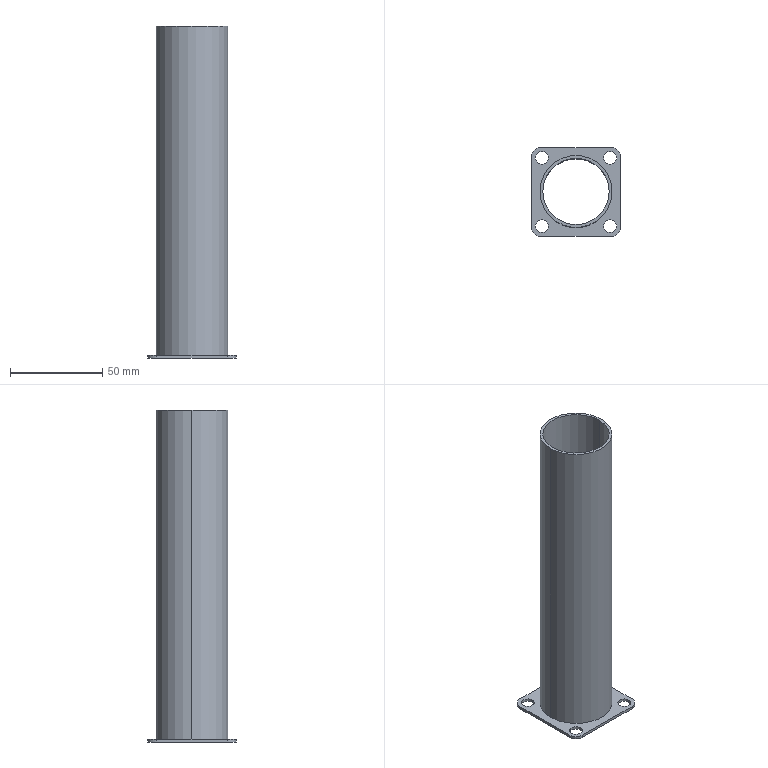Part | SolidWorks | features BaseBody 1 | 1 solid | 23 faces | box 48 x 48 x 180 mm | volume 33210 mm3 | cylinder 16 | plane 7 | commonest cylinder face diameters 7 x8 10 x4 36 x2 39 x2
STEP:
#1=CARTESIAN_POINT('',(-711.131,662.711,833.732));
#2=VERTEX_POINT('',#1);
#3=CARTESIAN_POINT('',(-711.131,662.711,832.232));
#4=VERTEX_POINT('',#3);
#5=CARTESIAN_POINT('',(-711.131,662.711,833.732));
#6=DIRECTION('',(0.,0.,-1.));
#7=VECTOR('',#6,1000.);
#8=LINE('',#5,#7);
#9=EDGE_CURVE('',#2,#4,#8,.T.);
#10=ORIENTED_EDGE('',*,*,#9,.F.);
#11=CARTESIAN_POINT('',(-718.131,662.711,833.732));
#12=VERTEX_POINT('',#11);
#13=CARTESIAN_POINT('',(-714.631,662.711,833.732));
#14=DIRECTION('',(0.,0.,1.));
#15=DIRECTION('',(1.,0.,0.));
#16=AXIS2_PLACEMENT_3D('',#13,#14,#15);
#17=CIRCLE('',#16,3.5);
#18=EDGE_CURVE('',#2,#12,#17,.T.);
#19=ORIENTED_EDGE('',*,*,#18,.T.);
#20=CARTESIAN_POINT('',(-718.131,662.711,832.232));
#21=VERTEX_POINT('',#20);
#22=CARTESIAN_POINT('',(-718.131,662.711,832.232));
#23=DIRECTION('',(0.,0.,1.));
#24=VECTOR('',#23,1000.);
#25=LINE('',#22,#24);
#26=EDGE_CURVE('',#21,#12,#25,.T.);
#27=ORIENTED_EDGE('',*,*,#26,.F.);
#28=CARTESIAN_POINT('',(-714.631,662.711,832.232));
#29=DIRECTION('',(0.,0.,-1.));
#30=DIRECTION('',(-1.,0.,0.));
#31=AXIS2_PLACEMENT_3D('',#28,#29,#30);
#32=CIRCLE('',#31,3.5);
#33=EDGE_CURVE('',#21,#4,#32,.T.);
#34=ORIENTED_EDGE('',*,*,#33,.T.);
#35=EDGE_LOOP('',(#10,#19,#27,#34));
#36=FACE_OUTER_BOUND('',#35,.T.);
#37=CARTESIAN_POINT('',(-714.631,662.711,833.732));
#38=DIRECTION('',(0.,0.,1.));
#39=DIRECTION('',(-1.,0.,0.));
#40=AXIS2_PLACEMENT_3D('',#37,#38,#39);
#41=CYLINDRICAL_SURFACE('',#40,3.5);
#42=ADVANCED_FACE('',(#36),#41,.F.);
#43=CARTESIAN_POINT('',(-757.131,700.211,832.232));
#44=VERTEX_POINT('',#43);
#45=CARTESIAN_POINT('',(-757.131,662.211,832.232));
#46=VERTEX_POINT('',#45);
#47=CARTESIAN_POINT('',(-757.131,700.211,832.232));
#48=DIRECTION('',(0.,-1.,0.));
#49=VECTOR('',#48,1000.);
#50=LINE('',#47,#49);
#51=EDGE_CURVE('',#44,#46,#50,.T.);
#52=ORIENTED_EDGE('',*,*,#51,.F.);
#53=CARTESIAN_POINT('',(-752.131,705.211,832.232));
#54=VERTEX_POINT('',#53);
#55=CARTESIAN_POINT('',(-752.131,700.211,832.232));
#56=DIRECTION('',(0.,0.,1.));
#57=DIRECTION('',(0.,1.,0.));
#58=AXIS2_PLACEMENT_3D('',#55,#56,#57);
#59=CIRCLE('',#58,5.);
#60=EDGE_CURVE('',#54,#44,#59,.T.);
#61=ORIENTED_EDGE('',*,*,#60,.F.);
#62=CARTESIAN_POINT('',(-714.131,705.211,832.232));
#63=VERTEX_POINT('',#62);
#64=CARTESIAN_POINT('',(-714.131,705.211,832.232));
#65=DIRECTION('',(-1.,0.,0.));
#66=VECTOR('',#65,1000.);
#67=LINE('',#64,#66);
#68=EDGE_CURVE('',#63,#54,#67,.T.);
#69=ORIENTED_EDGE('',*,*,#68,.F.);
#70=CARTESIAN_POINT('',(-709.131,700.211,832.232));
#71=VERTEX_POINT('',#70);
#72=CARTESIAN_POINT('',(-714.131,700.211,832.232));
#73=DIRECTION('',(0.,0.,1.));
#74=DIRECTION('',(1.,0.,0.));
#75=AXIS2_PLACEMENT_3D('',#72,#73,#74);
#76=CIRCLE('',#75,5.);
#77=EDGE_CURVE('',#71,#63,#76,.T.);
#78=ORIENTED_EDGE('',*,*,#77,.F.);
#79=CARTESIAN_POINT('',(-709.131,662.211,832.232));
#80=VERTEX_POINT('',#79);
#81=CARTESIAN_POINT('',(-709.131,662.211,832.232));
#82=DIRECTION('',(0.,1.,0.));
#83=VECTOR('',#82,1000.);
#84=LINE('',#81,#83);
#85=EDGE_CURVE('',#80,#71,#84,.T.);
#86=ORIENTED_EDGE('',*,*,#85,.F.);
#87=CARTESIAN_POINT('',(-714.131,657.211,832.232));
#88=VERTEX_POINT('',#87);
#89=CARTESIAN_POINT('',(-714.131,662.211,832.232));
#90=DIRECTION('',(0.,0.,1.));
#91=DIRECTION('',(0.,-1.,0.));
#92=AXIS2_PLACEMENT_3D('',#89,#90,#91);
#93=CIRCLE('',#92,5.);
#94=EDGE_CURVE('',#88,#80,#93,.T.);
#95=ORIENTED_EDGE('',*,*,#94,.F.);
#96=CARTESIAN_POINT('',(-752.131,657.211,832.232));
#97=VERTEX_POINT('',#96);
#98=CARTESIAN_POINT('',(-752.131,657.211,832.232));
#99=DIRECTION('',(1.,0.,0.));
#100=VECTOR('',#99,1000.);
#101=LINE('',#98,#100);
#102=EDGE_CURVE('',#97,#88,#101,.T.);
#103=ORIENTED_EDGE('',*,*,#102,.F.);
#104=CARTESIAN_POINT('',(-752.131,662.211,832.232));
#105=DIRECTION('',(0.,0.,1.));
#106=DIRECTION('',(-1.,0.,0.));
#107=AXIS2_PLACEMENT_3D('',#104,#105,#106);
#108=CIRCLE('',#107,5.);
#109=EDGE_CURVE('',#46,#97,#108,.T.);
#110=ORIENTED_EDGE('',*,*,#109,.F.);
#111=EDGE_LOOP('',(#52,#61,#69,#78,#86,#95,#103,#110));
#112=FACE_OUTER_BOUND('',#111,.T.);
#113=CARTESIAN_POINT('',(-748.131,662.711,832.232));
#114=VERTEX_POINT('',#113);
#115=CARTESIAN_POINT('',(-755.131,662.711,832.232));
#116=VERTEX_POINT('',#115);
#117=CARTESIAN_POINT('',(-751.631,662.711,832.232));
#118=DIRECTION('',(0.,0.,-1.));
#119=DIRECTION('',(1.,0.,0.));
#120=AXIS2_PLACEMENT_3D('',#117,#118,#119);
#121=CIRCLE('',#120,3.5);
#122=EDGE_CURVE('',#114,#116,#121,.T.);
#123=ORIENTED_EDGE('',*,*,#122,.F.);
#124=CARTESIAN_POINT('',(-751.631,662.711,832.232));
#125=DIRECTION('',(0.,0.,-1.));
#126=DIRECTION('',(-1.,0.,0.));
#127=AXIS2_PLACEMENT_3D('',#124,#125,#126);
#128=CIRCLE('',#127,3.5);
#129=EDGE_CURVE('',#116,#114,#128,.T.);
#130=ORIENTED_EDGE('',*,*,#129,.F.);
#131=EDGE_LOOP('',(#123,#130));
#132=FACE_BOUND('',#131,.T.);
#133=CARTESIAN_POINT('',(-748.131,699.711,832.232));
#134=VERTEX_POINT('',#133);
#135=CARTESIAN_POINT('',(-755.131,699.711,832.232));
#136=VERTEX_POINT('',#135);
#137=CARTESIAN_POINT('',(-751.631,699.711,832.232));
#138=DIRECTION('',(0.,0.,-1.));
#139=DIRECTION('',(1.,0.,0.));
#140=AXIS2_PLACEMENT_3D('',#137,#138,#139);
#141=CIRCLE('',#140,3.5);
#142=EDGE_CURVE('',#134,#136,#141,.T.);
#143=ORIENTED_EDGE('',*,*,#142,.F.);
#144=CARTESIAN_POINT('',(-751.631,699.711,832.232));
#145=DIRECTION('',(0.,0.,-1.));
#146=DIRECTION('',(-1.,0.,0.));
#147=AXIS2_PLACEMENT_3D('',#144,#145,#146);
#148=CIRCLE('',#147,3.5);
#149=EDGE_CURVE('',#136,#134,#148,.T.);
#150=ORIENTED_EDGE('',*,*,#149,.F.);
#151=EDGE_LOOP('',(#143,#150));
#152=FACE_BOUND('',#151,.T.);
#153=CARTESIAN_POINT('',(-714.631,662.711,832.232));
#154=DIRECTION('',(0.,0.,-1.));
#155=DIRECTION('',(1.,0.,0.));
#156=AXIS2_PLACEMENT_3D('',#153,#154,#155);
#157=CIRCLE('',#156,3.5);
#158=EDGE_CURVE('',#4,#21,#157,.T.);
#159=ORIENTED_EDGE('',*,*,#158,.F.);
#160=ORIENTED_EDGE('',*,*,#33,.F.);
#161=EDGE_LOOP('',(#159,#160));
#162=FACE_BOUND('',#161,.T.);
#163=CARTESIAN_POINT('',(-711.131,699.711,832.232));
#164=VERTEX_POINT('',#163);
#165=CARTESIAN_POINT('',(-718.131,699.711,832.232));
#166=VERTEX_POINT('',#165);
#167=CARTESIAN_POINT('',(-714.631,699.711,832.232));
#168=DIRECTION('',(0.,0.,-1.));
#169=DIRECTION('',(1.,0.,0.));
#170=AXIS2_PLACEMENT_3D('',#167,#168,#169);
#171=CIRCLE('',#170,3.5);
#172=EDGE_CURVE('',#164,#166,#171,.T.);
#173=ORIENTED_EDGE('',*,*,#172,.F.);
#174=CARTESIAN_POINT('',(-714.631,699.711,832.232));
#175=DIRECTION('',(0.,0.,-1.));
#176=DIRECTION('',(-1.,0.,0.));
#177=AXIS2_PLACEMENT_3D('',#174,#175,#176);
#178=CIRCLE('',#177,3.5);
#179=EDGE_CURVE('',#166,#164,#178,.T.);
#180=ORIENTED_EDGE('',*,*,#179,.F.);
#181=EDGE_LOOP('',(#173,#180));
#182=FACE_BOUND('',#181,.T.);
#183=CARTESIAN_POINT('',(-751.131,681.211,832.232));
#184=VERTEX_POINT('',#183);
#185=CARTESIAN_POINT('',(-715.131,681.211,832.232));
#186=VERTEX_POINT('',#185);
#187=CARTESIAN_POINT('',(-733.131,681.211,832.232));
#188=DIRECTION('',(0.,0.,-1.));
#189=DIRECTION('',(-1.,0.,0.));
#190=AXIS2_PLACEMENT_3D('',#187,#188,#189);
#191=CIRCLE('',#190,18.);
#192=EDGE_CURVE('',#184,#186,#191,.T.);
#193=ORIENTED_EDGE('',*,*,#192,.F.);
#194=CARTESIAN_POINT('',(-733.131,681.211,832.232));
#195=DIRECTION('',(0.,0.,-1.));
#196=DIRECTION('',(1.,0.,0.));
#197=AXIS2_PLACEMENT_3D('',#194,#195,#196);
#198=CIRCLE('',#197,18.);
#199=EDGE_CURVE('',#186,#184,#198,.T.);
#200=ORIENTED_EDGE('',*,*,#199,.F.);
#201=EDGE_LOOP('',(#193,#200));
#202=FACE_BOUND('',#201,.T.);
#203=CARTESIAN_POINT('',(-733.131,681.211,832.232));
#204=DIRECTION('',(0.,0.,-1.));
#205=DIRECTION('',(1.,0.,0.));
#206=AXIS2_PLACEMENT_3D('',#203,#204,#205);
#207=PLANE('',#206);
#208=ADVANCED_FACE('',(#112,#132,#152,#162,#182,#202),#207,.T.);
#209=CARTESIAN_POINT('',(-752.131,657.211,833.732));
#210=VERTEX_POINT('',#209);
#211=CARTESIAN_POINT('',(-757.131,662.211,833.732));
#212=VERTEX_POINT('',#211);
#213=CARTESIAN_POINT('',(-752.131,662.211,833.732));
#214=DIRECTION('',(0.,0.,-1.));
#215=DIRECTION('',(0.,-1.,0.));
#216=AXIS2_PLACEMENT_3D('',#213,#214,#215);
#217=CIRCLE('',#216,5.);
#218=EDGE_CURVE('',#210,#212,#217,.T.);
#219=ORIENTED_EDGE('',*,*,#218,.T.);
#220=CARTESIAN_POINT('',(-757.131,662.211,832.232));
#221=DIRECTION('',(0.,0.,1.));
#222=VECTOR('',#221,1000.);
#223=LINE('',#220,#222);
#224=EDGE_CURVE('',#46,#212,#223,.T.);
#225=ORIENTED_EDGE('',*,*,#224,.F.);
#226=ORIENTED_EDGE('',*,*,#109,.T.);
#227=CARTESIAN_POINT('',(-752.131,657.211,833.732));
#228=DIRECTION('',(0.,0.,-1.));
#229=VECTOR('',#228,1000.);
#230=LINE('',#227,#229);
#231=EDGE_CURVE('',#210,#97,#230,.T.);
#232=ORIENTED_EDGE('',*,*,#231,.F.);
#233=EDGE_LOOP('',(#219,#225,#226,#232));
#234=FACE_OUTER_BOUND('',#233,.T.);
#235=CARTESIAN_POINT('',(-752.131,662.211,832.232));
#236=DIRECTION('',(0.,0.,1.));
#237=DIRECTION('',(-1.,0.,0.));
#238=AXIS2_PLACEMENT_3D('',#235,#236,#237);
#239=CYLINDRICAL_SURFACE('',#238,5.);
#240=ADVANCED_FACE('',(#234),#239,.T.);
#241=ORIENTED_EDGE('',*,*,#102,.T.);
#242=CARTESIAN_POINT('',(-714.131,657.211,833.732));
#243=VERTEX_POINT('',#242);
#244=CARTESIAN_POINT('',(-714.131,657.211,832.232));
#245=DIRECTION('',(0.,0.,1.));
#246=VECTOR('',#245,1000.);
#247=LINE('',#244,#246);
#248=EDGE_CURVE('',#88,#243,#247,.T.);
#249=ORIENTED_EDGE('',*,*,#248,.T.);
#250=CARTESIAN_POINT('',(-752.131,657.211,833.732));
#251=DIRECTION('',(1.,0.,0.));
#252=VECTOR('',#251,1000.);
#253=LINE('',#250,#252);
#254=EDGE_CURVE('',#210,#243,#253,.T.);
#255=ORIENTED_EDGE('',*,*,#254,.F.);
#256=ORIENTED_EDGE('',*,*,#231,.T.);
#257=EDGE_LOOP('',(#241,#249,#255,#256));
#258=FACE_OUTER_BOUND('',#257,.T.);
#259=CARTESIAN_POINT('',(-757.131,657.211,832.232));
#260=DIRECTION('',(0.,1.,0.));
#261=DIRECTION('',(1.,0.,0.));
#262=AXIS2_PLACEMENT_3D('',#259,#260,#261);
#263=PLANE('',#262);
#264=ADVANCED_FACE('',(#258),#263,.F.);
#265=ORIENTED_EDGE('',*,*,#254,.T.);
#266=CARTESIAN_POINT('',(-709.131,662.211,833.732));
#267=VERTEX_POINT('',#266);
#268=CARTESIAN_POINT('',(-714.131,662.211,833.732));
#269=DIRECTION('',(0.,0.,-1.));
#270=DIRECTION('',(1.,0.,0.));
#271=AXIS2_PLACEMENT_3D('',#268,#269,#270);
#272=CIRCLE('',#271,5.);
#273=EDGE_CURVE('',#267,#243,#272,.T.);
#274=ORIENTED_EDGE('',*,*,#273,.F.);
#275=CARTESIAN_POINT('',(-709.131,700.211,833.732));
#276=VERTEX_POINT('',#275);
#277=CARTESIAN_POINT('',(-709.131,700.211,833.732));
#278=DIRECTION('',(0.,-1.,0.));
#279=VECTOR('',#278,1000.);
#280=LINE('',#277,#279);
#281=EDGE_CURVE('',#276,#267,#280,.T.);
#282=ORIENTED_EDGE('',*,*,#281,.F.);
#283=CARTESIAN_POINT('',(-714.131,705.211,833.732));
#284=VERTEX_POINT('',#283);
#285=CARTESIAN_POINT('',(-714.131,700.211,833.732));
#286=DIRECTION('',(0.,0.,-1.));
#287=DIRECTION('',(0.,1.,0.));
#288=AXIS2_PLACEMENT_3D('',#285,#286,#287);
#289=CIRCLE('',#288,5.);
#290=EDGE_CURVE('',#284,#276,#289,.T.);
#291=ORIENTED_EDGE('',*,*,#290,.F.);
#292=CARTESIAN_POINT('',(-752.131,705.211,833.732));
#293=VERTEX_POINT('',#292);
#294=CARTESIAN_POINT('',(-752.131,705.211,833.732));
#295=DIRECTION('',(1.,0.,0.));
#296=VECTOR('',#295,1000.);
#297=LINE('',#294,#296);
#298=EDGE_CURVE('',#293,#284,#297,.T.);
#299=ORIENTED_EDGE('',*,*,#298,.F.);
#300=CARTESIAN_POINT('',(-757.131,700.211,833.732));
#301=VERTEX_POINT('',#300);
#302=CARTESIAN_POINT('',(-752.131,700.211,833.732));
#303=DIRECTION('',(0.,0.,-1.));
#304=DIRECTION('',(-1.,0.,0.));
#305=AXIS2_PLACEMENT_3D('',#302,#303,#304);
#306=CIRCLE('',#305,5.);
#307=EDGE_CURVE('',#301,#293,#306,.T.);
#308=ORIENTED_EDGE('',*,*,#307,.F.);
#309=CARTESIAN_POINT('',(-757.131,662.211,833.732));
#310=DIRECTION('',(0.,1.,0.));
#311=VECTOR('',#310,1000.);
#312=LINE('',#309,#311);
#313=EDGE_CURVE('',#212,#301,#312,.T.);
#314=ORIENTED_EDGE('',*,*,#313,.F.);
#315=ORIENTED_EDGE('',*,*,#218,.F.);
#316=EDGE_LOOP('',(#265,#274,#282,#291,#299,#308,#314,#315));
#317=FACE_OUTER_BOUND('',#316,.T.);
#318=CARTESIAN_POINT('',(-748.131,662.711,833.732));
#319=VERTEX_POINT('',#318);
#320=CARTESIAN_POINT('',(-755.131,662.711,833.732));
#321=VERTEX_POINT('',#320);
#322=CARTESIAN_POINT('',(-751.631,662.711,833.732));
#323=DIRECTION('',(0.,0.,1.));
#324=DIRECTION('',(1.,0.,0.));
#325=AXIS2_PLACEMENT_3D('',#322,#323,#324);
#326=CIRCLE('',#325,3.5);
#327=EDGE_CURVE('',#319,#321,#326,.T.);
#328=ORIENTED_EDGE('',*,*,#327,.F.);
#329=CARTESIAN_POINT('',(-751.631,662.711,833.732));
#330=DIRECTION('',(0.,0.,1.));
#331=DIRECTION('',(-1.,0.,0.));
#332=AXIS2_PLACEMENT_3D('',#329,#330,#331);
#333=CIRCLE('',#332,3.5);
#334=EDGE_CURVE('',#321,#319,#333,.T.);
#335=ORIENTED_EDGE('',*,*,#334,.F.);
#336=EDGE_LOOP('',(#328,#335));
#337=FACE_BOUND('',#336,.T.);
#338=CARTESIAN_POINT('',(-748.131,699.711,833.732));
#339=VERTEX_POINT('',#338);
#340=CARTESIAN_POINT('',(-755.131,699.711,833.732));
#341=VERTEX_POINT('',#340);
#342=CARTESIAN_POINT('',(-751.631,699.711,833.732));
#343=DIRECTION('',(0.,0.,1.));
#344=DIRECTION('',(1.,0.,0.));
#345=AXIS2_PLACEMENT_3D('',#342,#343,#344);
#346=CIRCLE('',#345,3.5);
#347=EDGE_CURVE('',#339,#341,#346,.T.);
#348=ORIENTED_EDGE('',*,*,#347,.F.);
#349=CARTESIAN_POINT('',(-751.631,699.711,833.732));
#350=DIRECTION('',(0.,0.,1.));
#351=DIRECTION('',(-1.,0.,0.));
#352=AXIS2_PLACEMENT_3D('',#349,#350,#351);
#353=CIRCLE('',#352,3.5);
#354=EDGE_CURVE('',#341,#339,#353,.T.);
#355=ORIENTED_EDGE('',*,*,#354,.F.);
#356=EDGE_LOOP('',(#348,#355));
#357=FACE_BOUND('',#356,.T.);
#358=ORIENTED_EDGE('',*,*,#18,.F.);
#359=CARTESIAN_POINT('',(-714.631,662.711,833.732));
#360=DIRECTION('',(0.,0.,1.));
#361=DIRECTION('',(-1.,0.,0.));
#362=AXIS2_PLACEMENT_3D('',#359,#360,#361);
#363=CIRCLE('',#362,3.5);
#364=EDGE_CURVE('',#12,#2,#363,.T.);
#365=ORIENTED_EDGE('',*,*,#364,.F.);
#366=EDGE_LOOP('',(#358,#365));
#367=FACE_BOUND('',#366,.T.);
#368=CARTESIAN_POINT('',(-711.131,699.711,833.732));
#369=VERTEX_POINT('',#368);
#370=CARTESIAN_POINT('',(-718.131,699.711,833.732));
#371=VERTEX_POINT('',#370);
#372=CARTESIAN_POINT('',(-714.631,699.711,833.732));
#373=DIRECTION('',(0.,0.,1.));
#374=DIRECTION('',(1.,0.,0.));
#375=AXIS2_PLACEMENT_3D('',#372,#373,#374);
#376=CIRCLE('',#375,3.5);
#377=EDGE_CURVE('',#369,#371,#376,.T.);
#378=ORIENTED_EDGE('',*,*,#377,.F.);
#379=CARTESIAN_POINT('',(-714.631,699.711,833.732));
#380=DIRECTION('',(0.,0.,1.));
#381=DIRECTION('',(-1.,0.,0.));
#382=AXIS2_PLACEMENT_3D('',#379,#380,#381);
#383=CIRCLE('',#382,3.5);
#384=EDGE_CURVE('',#371,#369,#383,.T.);
#385=ORIENTED_EDGE('',*,*,#384,.F.);
#386=EDGE_LOOP('',(#378,#385));
#387=FACE_BOUND('',#386,.T.);
#388=CARTESIAN_POINT('',(-713.631,681.211,833.732));
#389=VERTEX_POINT('',#388);
#390=CARTESIAN_POINT('',(-752.631,681.211,833.732));
#391=VERTEX_POINT('',#390);
#392=CARTESIAN_POINT('',(-733.131,681.211,833.732));
#393=DIRECTION('',(0.,0.,1.));
#394=DIRECTION('',(1.,0.,0.));
#395=AXIS2_PLACEMENT_3D('',#392,#393,#394);
#396=CIRCLE('',#395,19.5);
#397=EDGE_CURVE('',#389,#391,#396,.T.);
#398=ORIENTED_EDGE('',*,*,#397,.F.);
#399=CARTESIAN_POINT('',(-733.131,681.211,833.732));
#400=DIRECTION('',(0.,0.,1.));
#401=DIRECTION('',(-1.,0.,0.));
#402=AXIS2_PLACEMENT_3D('',#399,#400,#401);
#403=CIRCLE('',#402,19.5);
#404=EDGE_CURVE('',#391,#389,#403,.T.);
#405=ORIENTED_EDGE('',*,*,#404,.F.);
#406=EDGE_LOOP('',(#398,#405));
#407=FACE_BOUND('',#406,.T.);
#408=CARTESIAN_POINT('',(-733.131,681.211,833.732));
#409=DIRECTION('',(0.,0.,-1.));
#410=DIRECTION('',(1.,0.,0.));
#411=AXIS2_PLACEMENT_3D('',#408,#409,#410);
#412=PLANE('',#411);
#413=ADVANCED_FACE('',(#317,#337,#357,#367,#387,#407),#412,.F.);
#414=ORIENTED_EDGE('',*,*,#313,.T.);
#415=CARTESIAN_POINT('',(-757.131,700.211,833.732));
#416=DIRECTION('',(0.,0.,-1.));
#417=VECTOR('',#416,1000.);
#418=LINE('',#415,#417);
#419=EDGE_CURVE('',#301,#44,#418,.T.);
#420=ORIENTED_EDGE('',*,*,#419,.T.);
#421=ORIENTED_EDGE('',*,*,#51,.T.);
#422=ORIENTED_EDGE('',*,*,#224,.T.);
#423=EDGE_LOOP('',(#414,#420,#421,#422));
#424=FACE_OUTER_BOUND('',#423,.T.);
#425=CARTESIAN_POINT('',(-757.131,657.211,832.232));
#426=DIRECTION('',(1.,0.,0.));
#427=DIRECTION('',(0.,0.,1.));
#428=AXIS2_PLACEMENT_3D('',#425,#426,#427);
#429=PLANE('',#428);
#430=ADVANCED_FACE('',(#424),#429,.F.);
#431=ORIENTED_EDGE('',*,*,#307,.T.);
#432=CARTESIAN_POINT('',(-752.131,705.211,832.232));
#433=DIRECTION('',(0.,0.,1.));
#434=VECTOR('',#433,1000.);
#435=LINE('',#432,#434);
#436=EDGE_CURVE('',#54,#293,#435,.T.);
#437=ORIENTED_EDGE('',*,*,#436,.F.);
#438=ORIENTED_EDGE('',*,*,#60,.T.);
#439=ORIENTED_EDGE('',*,*,#419,.F.);
#440=EDGE_LOOP('',(#431,#437,#438,#439));
#441=FACE_OUTER_BOUND('',#440,.T.);
#442=CARTESIAN_POINT('',(-752.131,700.211,832.232));
#443=DIRECTION('',(0.,0.,1.));
#444=DIRECTION('',(-1.,0.,0.));
#445=AXIS2_PLACEMENT_3D('',#442,#443,#444);
#446=CYLINDRICAL_SURFACE('',#445,5.);
#447=ADVANCED_FACE('',(#441),#446,.T.);
#448=ORIENTED_EDGE('',*,*,#298,.T.);
#449=CARTESIAN_POINT('',(-714.131,705.211,833.732));
#450=DIRECTION('',(0.,0.,-1.));
#451=VECTOR('',#450,1000.);
#452=LINE('',#449,#451);
#453=EDGE_CURVE('',#284,#63,#452,.T.);
#454=ORIENTED_EDGE('',*,*,#453,.T.);
#455=ORIENTED_EDGE('',*,*,#68,.T.);
#456=ORIENTED_EDGE('',*,*,#436,.T.);
#457=EDGE_LOOP('',(#448,#454,#455,#456));
#458=FACE_OUTER_BOUND('',#457,.T.);
#459=CARTESIAN_POINT('',(-757.131,705.211,832.232));
#460=DIRECTION('',(0.,-1.,0.));
#461=DIRECTION('',(-1.,0.,0.));
#462=AXIS2_PLACEMENT_3D('',#459,#460,#461);
#463=PLANE('',#462);
#464=ADVANCED_FACE('',(#458),#463,.F.);
#465=ORIENTED_EDGE('',*,*,#290,.T.);
#466=CARTESIAN_POINT('',(-709.131,700.211,832.232));
#467=DIRECTION('',(0.,0.,1.));
#468=VECTOR('',#467,1000.);
#469=LINE('',#466,#468);
#470=EDGE_CURVE('',#71,#276,#469,.T.);
#471=ORIENTED_EDGE('',*,*,#470,.F.);
#472=ORIENTED_EDGE('',*,*,#77,.T.);
#473=ORIENTED_EDGE('',*,*,#453,.F.);
#474=EDGE_LOOP('',(#465,#471,#472,#473));
#475=FACE_OUTER_BOUND('',#474,.T.);
#476=CARTESIAN_POINT('',(-714.131,700.211,832.232));
#477=DIRECTION('',(0.,0.,1.));
#478=DIRECTION('',(-1.,0.,0.));
#479=AXIS2_PLACEMENT_3D('',#476,#477,#478);
#480=CYLINDRICAL_SURFACE('',#479,5.);
#481=ADVANCED_FACE('',(#475),#480,.T.);
#482=ORIENTED_EDGE('',*,*,#85,.T.);
#483=ORIENTED_EDGE('',*,*,#470,.T.);
#484=ORIENTED_EDGE('',*,*,#281,.T.);
#485=CARTESIAN_POINT('',(-709.131,662.211,833.732));
#486=DIRECTION('',(0.,0.,-1.));
#487=VECTOR('',#486,1000.);
#488=LINE('',#485,#487);
#489=EDGE_CURVE('',#267,#80,#488,.T.);
#490=ORIENTED_EDGE('',*,*,#489,.T.);
#491=EDGE_LOOP('',(#482,#483,#484,#490));
#492=FACE_OUTER_BOUND('',#491,.T.);
#493=CARTESIAN_POINT('',(-709.131,657.211,832.232));
#494=DIRECTION('',(-1.,0.,0.));
#495=DIRECTION('',(0.,0.,-1.));
#496=AXIS2_PLACEMENT_3D('',#493,#494,#495);
#497=PLANE('',#496);
#498=ADVANCED_FACE('',(#492),#497,.F.);
#499=ORIENTED_EDGE('',*,*,#273,.T.);
#500=ORIENTED_EDGE('',*,*,#248,.F.);
#501=ORIENTED_EDGE('',*,*,#94,.T.);
#502=ORIENTED_EDGE('',*,*,#489,.F.);
#503=EDGE_LOOP('',(#499,#500,#501,#502));
#504=FACE_OUTER_BOUND('',#503,.T.);
#505=CARTESIAN_POINT('',(-714.131,662.211,832.232));
#506=DIRECTION('',(0.,0.,1.));
#507=DIRECTION('',(-1.,0.,0.));
#508=AXIS2_PLACEMENT_3D('',#505,#506,#507);
#509=CYLINDRICAL_SURFACE('',#508,5.);
#510=ADVANCED_FACE('',(#504),#509,.T.);
#511=ORIENTED_EDGE('',*,*,#334,.T.);
#512=CARTESIAN_POINT('',(-748.131,662.711,833.732));
#513=DIRECTION('',(0.,0.,-1.));
#514=VECTOR('',#513,1000.);
#515=LINE('',#512,#514);
#516=EDGE_CURVE('',#319,#114,#515,.T.);
#517=ORIENTED_EDGE('',*,*,#516,.T.);
#518=ORIENTED_EDGE('',*,*,#122,.T.);
#519=CARTESIAN_POINT('',(-755.131,662.711,832.232));
#520=DIRECTION('',(0.,0.,1.));
#521=VECTOR('',#520,1000.);
#522=LINE('',#519,#521);
#523=EDGE_CURVE('',#116,#321,#522,.T.);
#524=ORIENTED_EDGE('',*,*,#523,.T.);
#525=EDGE_LOOP('',(#511,#517,#518,#524));
#526=FACE_OUTER_BOUND('',#525,.T.);
#527=CARTESIAN_POINT('',(-751.631,662.711,833.732));
#528=DIRECTION('',(0.,0.,1.));
#529=DIRECTION('',(-1.,0.,0.));
#530=AXIS2_PLACEMENT_3D('',#527,#528,#529);
#531=CYLINDRICAL_SURFACE('',#530,3.5);
#532=ADVANCED_FACE('',(#526),#531,.F.);
#533=ORIENTED_EDGE('',*,*,#516,.F.);
#534=ORIENTED_EDGE('',*,*,#327,.T.);
#535=ORIENTED_EDGE('',*,*,#523,.F.);
#536=ORIENTED_EDGE('',*,*,#129,.T.);
#537=EDGE_LOOP('',(#533,#534,#535,#536));
#538=FACE_OUTER_BOUND('',#537,.T.);
#539=CARTESIAN_POINT('',(-751.631,662.711,833.732));
#540=DIRECTION('',(0.,0.,1.));
#541=DIRECTION('',(-1.,0.,0.));
#542=AXIS2_PLACEMENT_3D('',#539,#540,#541);
#543=CYLINDRICAL_SURFACE('',#542,3.5);
#544=ADVANCED_FACE('',(#538),#543,.F.);
#545=ORIENTED_EDGE('',*,*,#354,.T.);
#546=CARTESIAN_POINT('',(-748.131,699.711,833.732));
#547=DIRECTION('',(0.,0.,-1.));
#548=VECTOR('',#547,1000.);
#549=LINE('',#546,#548);
#550=EDGE_CURVE('',#339,#134,#549,.T.);
#551=ORIENTED_EDGE('',*,*,#550,.T.);
#552=ORIENTED_EDGE('',*,*,#142,.T.);
#553=CARTESIAN_POINT('',(-755.131,699.711,832.232));
#554=DIRECTION('',(0.,0.,1.));
#555=VECTOR('',#554,1000.);
#556=LINE('',#553,#555);
#557=EDGE_CURVE('',#136,#341,#556,.T.);
#558=ORIENTED_EDGE('',*,*,#557,.T.);
#559=EDGE_LOOP('',(#545,#551,#552,#558));
#560=FACE_OUTER_BOUND('',#559,.T.);
#561=CARTESIAN_POINT('',(-751.631,699.711,833.732));
#562=DIRECTION('',(0.,0.,1.));
#563=DIRECTION('',(-1.,0.,0.));
#564=AXIS2_PLACEMENT_3D('',#561,#562,#563);
#565=CYLINDRICAL_SURFACE('',#564,3.5);
#566=ADVANCED_FACE('',(#560),#565,.F.);
#567=ORIENTED_EDGE('',*,*,#550,.F.);
#568=ORIENTED_EDGE('',*,*,#347,.T.);
#569=ORIENTED_EDGE('',*,*,#557,.F.);
#570=ORIENTED_EDGE('',*,*,#149,.T.);
#571=EDGE_LOOP('',(#567,#568,#569,#570));
#572=FACE_OUTER_BOUND('',#571,.T.);
#573=CARTESIAN_POINT('',(-751.631,699.711,833.732));
#574=DIRECTION('',(0.,0.,1.));
#575=DIRECTION('',(-1.,0.,0.));
#576=AXIS2_PLACEMENT_3D('',#573,#574,#575);
#577=CYLINDRICAL_SURFACE('',#576,3.5);
#578=ADVANCED_FACE('',(#572),#577,.F.);
#579=ORIENTED_EDGE('',*,*,#364,.T.);
#580=ORIENTED_EDGE('',*,*,#9,.T.);
#581=ORIENTED_EDGE('',*,*,#158,.T.);
#582=ORIENTED_EDGE('',*,*,#26,.T.);
#583=EDGE_LOOP('',(#579,#580,#581,#582));
#584=FACE_OUTER_BOUND('',#583,.T.);
#585=CARTESIAN_POINT('',(-714.631,662.711,833.732));
#586=DIRECTION('',(0.,0.,1.));
#587=DIRECTION('',(-1.,0.,0.));
#588=AXIS2_PLACEMENT_3D('',#585,#586,#587);
#589=CYLINDRICAL_SURFACE('',#588,3.5);
#590=ADVANCED_FACE('',(#584),#589,.F.);
#591=ORIENTED_EDGE('',*,*,#384,.T.);
#592=CARTESIAN_POINT('',(-711.131,699.711,833.732));
#593=DIRECTION('',(0.,0.,-1.));
#594=VECTOR('',#593,1000.);
#595=LINE('',#592,#594);
#596=EDGE_CURVE('',#369,#164,#595,.T.);
#597=ORIENTED_EDGE('',*,*,#596,.T.);
#598=ORIENTED_EDGE('',*,*,#172,.T.);
#599=CARTESIAN_POINT('',(-718.131,699.711,832.232));
#600=DIRECTION('',(0.,0.,1.));
#601=VECTOR('',#600,1000.);
#602=LINE('',#599,#601);
#603=EDGE_CURVE('',#166,#371,#602,.T.);
#604=ORIENTED_EDGE('',*,*,#603,.T.);
#605=EDGE_LOOP('',(#591,#597,#598,#604));
#606=FACE_OUTER_BOUND('',#605,.T.);
#607=CARTESIAN_POINT('',(-714.631,699.711,833.732));
#608=DIRECTION('',(0.,0.,1.));
#609=DIRECTION('',(-1.,0.,0.));
#610=AXIS2_PLACEMENT_3D('',#607,#608,#609);
#611=CYLINDRICAL_SURFACE('',#610,3.5);
#612=ADVANCED_FACE('',(#606),#611,.F.);
#613=ORIENTED_EDGE('',*,*,#596,.F.);
#614=ORIENTED_EDGE('',*,*,#377,.T.);
#615=ORIENTED_EDGE('',*,*,#603,.F.);
#616=ORIENTED_EDGE('',*,*,#179,.T.);
#617=EDGE_LOOP('',(#613,#614,#615,#616));
#618=FACE_OUTER_BOUND('',#617,.T.);
#619=CARTESIAN_POINT('',(-714.631,699.711,833.732));
#620=DIRECTION('',(0.,0.,1.));
#621=DIRECTION('',(-1.,0.,0.));
#622=AXIS2_PLACEMENT_3D('',#619,#620,#621);
#623=CYLINDRICAL_SURFACE('',#622,3.5);
#624=ADVANCED_FACE('',(#618),#623,.F.);
#625=CARTESIAN_POINT('',(-752.631,681.211,1012.232));
#626=VERTEX_POINT('',#625);
#627=CARTESIAN_POINT('',(-752.631,681.211,1012.232));
#628=DIRECTION('',(0.,0.,-1.));
#629=VECTOR('',#628,1000.);
#630=LINE('',#627,#629);
#631=EDGE_CURVE('',#626,#391,#630,.T.);
#632=ORIENTED_EDGE('',*,*,#631,.T.);
#633=ORIENTED_EDGE('',*,*,#404,.T.);
#634=CARTESIAN_POINT('',(-713.631,681.211,1012.232));
#635=VERTEX_POINT('',#634);
#636=CARTESIAN_POINT('',(-713.631,681.211,833.732));
#637=DIRECTION('',(0.,0.,1.));
#638=VECTOR('',#637,1000.);
#639=LINE('',#636,#638);
#640=EDGE_CURVE('',#389,#635,#639,.T.);
#641=ORIENTED_EDGE('',*,*,#640,.T.);
#642=CARTESIAN_POINT('',(-733.131,681.211,1012.232));
#643=DIRECTION('',(0.,0.,-1.));
#644=DIRECTION('',(1.,0.,0.));
#645=AXIS2_PLACEMENT_3D('',#642,#643,#644);
#646=CIRCLE('',#645,19.5);
#647=EDGE_CURVE('',#635,#626,#646,.T.);
#648=ORIENTED_EDGE('',*,*,#647,.T.);
#649=EDGE_LOOP('',(#632,#633,#641,#648));
#650=FACE_OUTER_BOUND('',#649,.T.);
#651=CARTESIAN_POINT('',(-733.131,681.211,1012.232));
#652=DIRECTION('',(0.,0.,-1.));
#653=DIRECTION('',(1.,0.,0.));
#654=AXIS2_PLACEMENT_3D('',#651,#652,#653);
#655=CYLINDRICAL_SURFACE('',#654,19.5);
#656=ADVANCED_FACE('',(#650),#655,.T.);
#657=ORIENTED_EDGE('',*,*,#647,.F.);
#658=CARTESIAN_POINT('',(-733.131,681.211,1012.232));
#659=DIRECTION('',(0.,0.,-1.));
#660=DIRECTION('',(-1.,0.,0.));
#661=AXIS2_PLACEMENT_3D('',#658,#659,#660);
#662=CIRCLE('',#661,19.5);
#663=EDGE_CURVE('',#626,#635,#662,.T.);
#664=ORIENTED_EDGE('',*,*,#663,.F.);
#665=EDGE_LOOP('',(#657,#664));
#666=FACE_OUTER_BOUND('',#665,.T.);
#667=CARTESIAN_POINT('',(-751.131,681.211,1012.232));
#668=VERTEX_POINT('',#667);
#669=CARTESIAN_POINT('',(-715.131,681.211,1012.232));
#670=VERTEX_POINT('',#669);
#671=CARTESIAN_POINT('',(-733.131,681.211,1012.232));
#672=DIRECTION('',(0.,0.,1.));
#673=DIRECTION('',(-1.,0.,0.));
#674=AXIS2_PLACEMENT_3D('',#671,#672,#673);
#675=CIRCLE('',#674,18.);
#676=EDGE_CURVE('',#668,#670,#675,.T.);
#677=ORIENTED_EDGE('',*,*,#676,.F.);
#678=CARTESIAN_POINT('',(-733.131,681.211,1012.232));
#679=DIRECTION('',(0.,0.,1.));
#680=DIRECTION('',(1.,0.,0.));
#681=AXIS2_PLACEMENT_3D('',#678,#679,#680);
#682=CIRCLE('',#681,18.);
#683=EDGE_CURVE('',#670,#668,#682,.T.);
#684=ORIENTED_EDGE('',*,*,#683,.F.);
#685=EDGE_LOOP('',(#677,#684));
#686=FACE_BOUND('',#685,.T.);
#687=CARTESIAN_POINT('',(-733.131,681.211,1012.232));
#688=DIRECTION('',(0.,0.,1.));
#689=DIRECTION('',(-1.,0.,0.));
#690=AXIS2_PLACEMENT_3D('',#687,#688,#689);
#691=PLANE('',#690);
#692=ADVANCED_FACE('',(#666,#686),#691,.T.);
#693=ORIENTED_EDGE('',*,*,#397,.T.);
#694=ORIENTED_EDGE('',*,*,#631,.F.);
#695=ORIENTED_EDGE('',*,*,#663,.T.);
#696=ORIENTED_EDGE('',*,*,#640,.F.);
#697=EDGE_LOOP('',(#693,#694,#695,#696));
#698=FACE_OUTER_BOUND('',#697,.T.);
#699=CARTESIAN_POINT('',(-733.131,681.211,1012.232));
#700=DIRECTION('',(0.,0.,-1.));
#701=DIRECTION('',(1.,0.,0.));
#702=AXIS2_PLACEMENT_3D('',#699,#700,#701);
#703=CYLINDRICAL_SURFACE('',#702,19.5);
#704=ADVANCED_FACE('',(#698),#703,.T.);
#705=CARTESIAN_POINT('',(-751.131,681.211,1012.232));
#706=DIRECTION('',(0.,0.,-1.));
#707=VECTOR('',#706,1000.);
#708=LINE('',#705,#707);
#709=EDGE_CURVE('',#668,#184,#708,.T.);
#710=ORIENTED_EDGE('',*,*,#709,.T.);
#711=ORIENTED_EDGE('',*,*,#192,.T.);
#712=CARTESIAN_POINT('',(-715.131,681.211,832.232));
#713=DIRECTION('',(0.,0.,1.));
#714=VECTOR('',#713,1000.);
#715=LINE('',#712,#714);
#716=EDGE_CURVE('',#186,#670,#715,.T.);
#717=ORIENTED_EDGE('',*,*,#716,.T.);
#718=ORIENTED_EDGE('',*,*,#683,.T.);
#719=EDGE_LOOP('',(#710,#711,#717,#718));
#720=FACE_OUTER_BOUND('',#719,.T.);
#721=CARTESIAN_POINT('',(-733.131,681.211,1012.232));
#722=DIRECTION('',(0.,0.,-1.));
#723=DIRECTION('',(1.,0.,0.));
#724=AXIS2_PLACEMENT_3D('',#721,#722,#723);
#725=CYLINDRICAL_SURFACE('',#724,18.);
#726=ADVANCED_FACE('',(#720),#725,.F.);
#727=ORIENTED_EDGE('',*,*,#199,.T.);
#728=ORIENTED_EDGE('',*,*,#709,.F.);
#729=ORIENTED_EDGE('',*,*,#676,.T.);
#730=ORIENTED_EDGE('',*,*,#716,.F.);
#731=EDGE_LOOP('',(#727,#728,#729,#730));
#732=FACE_OUTER_BOUND('',#731,.T.);
#733=CARTESIAN_POINT('',(-733.131,681.211,1012.232));
#734=DIRECTION('',(0.,0.,-1.));
#735=DIRECTION('',(1.,0.,0.));
#736=AXIS2_PLACEMENT_3D('',#733,#734,#735);
#737=CYLINDRICAL_SURFACE('',#736,18.);
#738=ADVANCED_FACE('',(#732),#737,.F.);
#739=CLOSED_SHELL('',(#42,#208,#240,#264,#413,#430,#447,#464,#481,#498,#510,#532,#544,#566,#578,#590,#612,#624,#656,#692,#704,#726,#738));
#740=MANIFOLD_SOLID_BREP('',#739);
#741=CARTESIAN_POINT('',(0.,0.,0.));
#742=DIRECTION('',(0.,0.,1.));
#743=DIRECTION('',(1.,0.,0.));
#744=AXIS2_PLACEMENT_3D('',#741,#742,#743);
#745=(LENGTH_UNIT()NAMED_UNIT(*)SI_UNIT(.MILLI.,.METRE.));
#746=UNCERTAINTY_MEASURE_WITH_UNIT(LENGTH_MEASURE(0.00001),#745,'','');
#747=(NAMED_UNIT(*)PLANE_ANGLE_UNIT()SI_UNIT($,.RADIAN.));
#748=(NAMED_UNIT(*)SI_UNIT($,.STERADIAN.)SOLID_ANGLE_UNIT());
#749=(GEOMETRIC_REPRESENTATION_CONTEXT(3)GLOBAL_UNCERTAINTY_ASSIGNED_CONTEXT((#746))GLOBAL_UNIT_ASSIGNED_CONTEXT((#745,#747,#748))REPRESENTATION_CONTEXT('',''));
#750=ADVANCED_BREP_SHAPE_REPRESENTATION('',(#740,#744),#749);